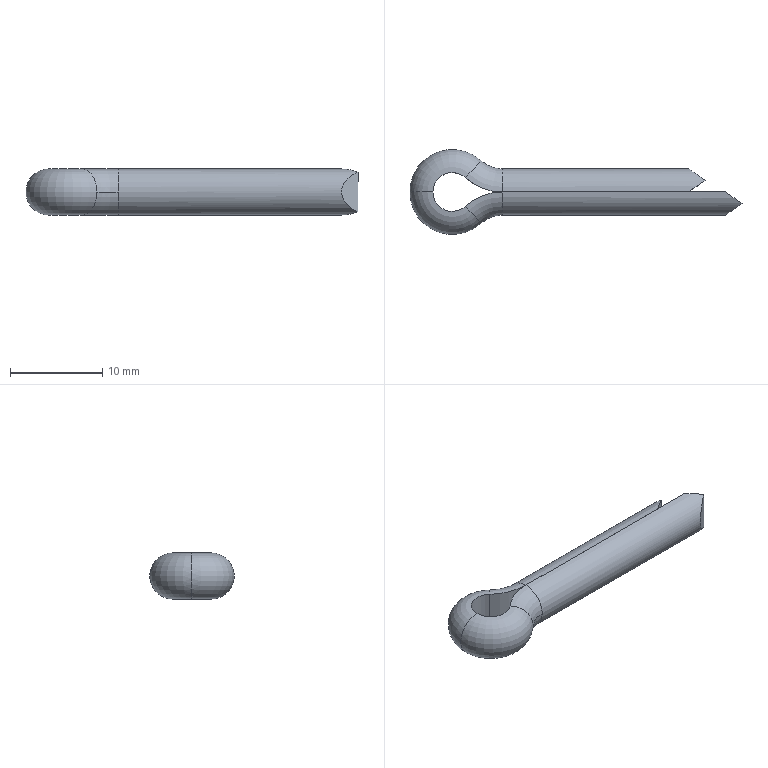Part | SolidWorks | features Cut 1, Sweep 1 | 1 solid | 17 faces | box 36 x 9.2 x 5 mm | volume 667.949 mm3 | torus 6 | plane 6 | cylinder 5 | commonest cylinder face diameters 5 x2 11.782 x2 4.204 x1
STEP:
#1=CARTESIAN_POINT('',(0.,2.5,0.));
#2=VERTEX_POINT('',#1);
#3=CARTESIAN_POINT('',(0.,0.002,2.5));
#4=VERTEX_POINT('',#3);
#5=CARTESIAN_POINT('',(0.,0.,0.));
#6=DIRECTION('',(1.,0.,0.));
#7=DIRECTION('',(0.,0.,-1.));
#8=AXIS2_PLACEMENT_3D('',#5,#6,#7);
#9=CIRCLE('',#8,2.5);
#10=EDGE_CURVE('',#2,#4,#9,.T.);
#11=ORIENTED_EDGE('',*,*,#10,.F.);
#12=CARTESIAN_POINT('',(-2.292,3.391,0.));
#13=VERTEX_POINT('',#12);
#14=CARTESIAN_POINT('',(0.,5.893,0.));
#15=DIRECTION('',(0.,0.,-1.));
#16=DIRECTION('',(-1.,0.,0.));
#17=AXIS2_PLACEMENT_3D('',#14,#15,#16);
#18=CIRCLE('',#17,3.393);
#19=EDGE_CURVE('',#2,#13,#18,.T.);
#20=ORIENTED_EDGE('',*,*,#19,.T.);
#21=CARTESIAN_POINT('',(-3.98,1.55,2.5));
#22=VERTEX_POINT('',#21);
#23=CARTESIAN_POINT('',(-3.981,1.548,0.));
#24=DIRECTION('',(0.7373,-0.6756,0.));
#25=DIRECTION('',(0.,0.,-1.));
#26=AXIS2_PLACEMENT_3D('',#23,#24,#25);
#27=CIRCLE('',#26,2.5);
#28=EDGE_CURVE('',#13,#22,#27,.T.);
#29=ORIENTED_EDGE('',*,*,#28,.T.);
#30=CARTESIAN_POINT('',(0.,5.893,2.5));
#31=DIRECTION('',(0.,0.,-1.));
#32=DIRECTION('',(-1.,0.,0.));
#33=AXIS2_PLACEMENT_3D('',#30,#31,#32);
#34=CIRCLE('',#33,5.891);
#35=EDGE_CURVE('',#4,#22,#34,.T.);
#36=ORIENTED_EDGE('',*,*,#35,.F.);
#37=EDGE_LOOP('',(#11,#20,#29,#36));
#38=FACE_OUTER_BOUND('',#37,.T.);
#39=CARTESIAN_POINT('',(0.,5.893,0.));
#40=DIRECTION('',(0.,0.,-1.));
#41=DIRECTION('',(-1.,0.,0.));
#42=AXIS2_PLACEMENT_3D('',#39,#40,#41);
#43=TOROIDAL_SURFACE('',#42,5.893,2.5);
#44=ADVANCED_FACE('',(#38),#43,.T.);
#45=CARTESIAN_POINT('',(-2.292,-3.391,0.));
#46=VERTEX_POINT('',#45);
#47=CARTESIAN_POINT('',(-3.98,-1.55,2.5));
#48=VERTEX_POINT('',#47);
#49=CARTESIAN_POINT('',(-3.981,-1.548,0.));
#50=DIRECTION('',(-0.7373,-0.6756,0.));
#51=DIRECTION('',(0.,0.,-1.));
#52=AXIS2_PLACEMENT_3D('',#49,#50,#51);
#53=CIRCLE('',#52,2.5);
#54=EDGE_CURVE('',#46,#48,#53,.T.);
#55=ORIENTED_EDGE('',*,*,#54,.F.);
#56=CARTESIAN_POINT('',(0.,-2.5,0.));
#57=VERTEX_POINT('',#56);
#58=CARTESIAN_POINT('',(0.,-5.893,0.));
#59=DIRECTION('',(0.,0.,-1.));
#60=DIRECTION('',(-1.,0.,0.));
#61=AXIS2_PLACEMENT_3D('',#58,#59,#60);
#62=CIRCLE('',#61,3.393);
#63=EDGE_CURVE('',#46,#57,#62,.T.);
#64=ORIENTED_EDGE('',*,*,#63,.T.);
#65=CARTESIAN_POINT('',(0.,-0.002,2.5));
#66=VERTEX_POINT('',#65);
#67=CARTESIAN_POINT('',(0.,0.,0.));
#68=DIRECTION('',(-1.,0.,0.));
#69=DIRECTION('',(0.,0.,-1.));
#70=AXIS2_PLACEMENT_3D('',#67,#68,#69);
#71=CIRCLE('',#70,2.5);
#72=EDGE_CURVE('',#57,#66,#71,.T.);
#73=ORIENTED_EDGE('',*,*,#72,.T.);
#74=CARTESIAN_POINT('',(0.,-5.893,2.5));
#75=DIRECTION('',(0.,0.,-1.));
#76=DIRECTION('',(-1.,0.,0.));
#77=AXIS2_PLACEMENT_3D('',#74,#75,#76);
#78=CIRCLE('',#77,5.891);
#79=EDGE_CURVE('',#48,#66,#78,.T.);
#80=ORIENTED_EDGE('',*,*,#79,.F.);
#81=EDGE_LOOP('',(#55,#64,#73,#80));
#82=FACE_OUTER_BOUND('',#81,.T.);
#83=CARTESIAN_POINT('',(0.,-5.893,0.));
#84=DIRECTION('',(0.,0.,-1.));
#85=DIRECTION('',(-1.,0.,0.));
#86=AXIS2_PLACEMENT_3D('',#83,#84,#85);
#87=TOROIDAL_SURFACE('',#86,5.893,2.5);
#88=ADVANCED_FACE('',(#82),#87,.T.);
#89=CARTESIAN_POINT('',(-3.98,1.55,-2.5));
#90=VERTEX_POINT('',#89);
#91=CARTESIAN_POINT('',(-7.502,0.,-2.5));
#92=VERTEX_POINT('',#91);
#93=CARTESIAN_POINT('',(-5.4,0.,-2.5));
#94=DIRECTION('',(0.,0.,1.));
#95=DIRECTION('',(1.,0.,0.));
#96=AXIS2_PLACEMENT_3D('',#93,#94,#95);
#97=CIRCLE('',#96,2.102);
#98=EDGE_CURVE('',#90,#92,#97,.T.);
#99=ORIENTED_EDGE('',*,*,#98,.T.);
#100=CARTESIAN_POINT('',(-7.502,0.,2.5));
#101=VERTEX_POINT('',#100);
#102=CARTESIAN_POINT('',(-7.5,0.,0.));
#103=DIRECTION('',(0.,1.,0.));
#104=DIRECTION('',(-1.,0.,0.));
#105=AXIS2_PLACEMENT_3D('',#102,#103,#104);
#106=CIRCLE('',#105,2.5);
#107=EDGE_CURVE('',#92,#101,#106,.T.);
#108=ORIENTED_EDGE('',*,*,#107,.T.);
#109=CARTESIAN_POINT('',(-5.4,0.,2.5));
#110=DIRECTION('',(0.,0.,1.));
#111=DIRECTION('',(1.,0.,0.));
#112=AXIS2_PLACEMENT_3D('',#109,#110,#111);
#113=CIRCLE('',#112,2.102);
#114=EDGE_CURVE('',#22,#101,#113,.T.);
#115=ORIENTED_EDGE('',*,*,#114,.F.);
#116=ORIENTED_EDGE('',*,*,#28,.F.);
#117=CARTESIAN_POINT('',(-3.981,1.548,0.));
#118=DIRECTION('',(0.7373,-0.6756,0.));
#119=DIRECTION('',(0.,0.,-1.));
#120=AXIS2_PLACEMENT_3D('',#117,#118,#119);
#121=CIRCLE('',#120,2.5);
#122=EDGE_CURVE('',#90,#13,#121,.T.);
#123=ORIENTED_EDGE('',*,*,#122,.F.);
#124=EDGE_LOOP('',(#99,#108,#115,#116,#123));
#125=FACE_OUTER_BOUND('',#124,.T.);
#126=CARTESIAN_POINT('',(-5.4,0.,0.));
#127=DIRECTION('',(0.,0.,1.));
#128=DIRECTION('',(1.,0.,0.));
#129=AXIS2_PLACEMENT_3D('',#126,#127,#128);
#130=TOROIDAL_SURFACE('',#129,2.1,2.5);
#131=ADVANCED_FACE('',(#125),#130,.T.);
#132=CARTESIAN_POINT('',(24.208,-0.002,2.5));
#133=VERTEX_POINT('',#132);
#134=CARTESIAN_POINT('',(0.,-0.002,2.5));
#135=DIRECTION('',(1.,0.,0.));
#136=VECTOR('',#135,1000.);
#137=LINE('',#134,#136);
#138=EDGE_CURVE('',#66,#133,#137,.T.);
#139=ORIENTED_EDGE('',*,*,#138,.T.);
#140=CARTESIAN_POINT('',(24.208,-0.002,-2.5));
#141=VERTEX_POINT('',#140);
#142=CARTESIAN_POINT('',(24.208,-0.002,2.5));
#143=DIRECTION('',(0.,0.,-1.));
#144=VECTOR('',#143,1000.);
#145=LINE('',#142,#144);
#146=EDGE_CURVE('',#133,#141,#145,.T.);
#147=ORIENTED_EDGE('',*,*,#146,.T.);
#148=CARTESIAN_POINT('',(0.,-0.002,-2.5));
#149=VERTEX_POINT('',#148);
#150=CARTESIAN_POINT('',(0.,-0.002,-2.5));
#151=DIRECTION('',(1.,0.,0.));
#152=VECTOR('',#151,1000.);
#153=LINE('',#150,#152);
#154=EDGE_CURVE('',#149,#141,#153,.T.);
#155=ORIENTED_EDGE('',*,*,#154,.F.);
#156=CARTESIAN_POINT('',(0.,-0.002,2.5));
#157=DIRECTION('',(0.,0.,-1.));
#158=VECTOR('',#157,1000.);
#159=LINE('',#156,#158);
#160=EDGE_CURVE('',#66,#149,#159,.T.);
#161=ORIENTED_EDGE('',*,*,#160,.F.);
#162=EDGE_LOOP('',(#139,#147,#155,#161));
#163=FACE_OUTER_BOUND('',#162,.T.);
#164=CARTESIAN_POINT('',(0.,-0.002,2.5));
#165=DIRECTION('',(0.,-1.,0.));
#166=DIRECTION('',(1.,0.,0.));
#167=AXIS2_PLACEMENT_3D('',#164,#165,#166);
#168=PLANE('',#167);
#169=ADVANCED_FACE('',(#163),#168,.F.);
#170=CARTESIAN_POINT('',(26.,-1.251,-2.164));
#171=VERTEX_POINT('',#170);
#172=CARTESIAN_POINT('',(26.,-1.251,2.164));
#173=VERTEX_POINT('',#172);
#174=CARTESIAN_POINT('',(26.,-1.251,-2.164));
#175=CARTESIAN_POINT('',(23.337,-3.124,-1.082));
#176=CARTESIAN_POINT('',(23.337,-3.124,1.082));
#177=CARTESIAN_POINT('',(26.,-1.251,2.164));
#178=(BOUNDED_CURVE()B_SPLINE_CURVE(3,(#174,#175,#176,#177),.UNSPECIFIED.,.F.,.T.)B_SPLINE_CURVE_WITH_KNOTS((4,4),(2.095,4.188),.UNSPECIFIED.)CURVE()GEOMETRIC_REPRESENTATION_ITEM()RATIONAL_B_SPLINE_CURVE((1.,0.6669,0.6669,1.))REPRESENTATION_ITEM(''));
#179=EDGE_CURVE('',#171,#173,#178,.T.);
#180=ORIENTED_EDGE('',*,*,#179,.T.);
#181=CARTESIAN_POINT('',(26.,-1.251,2.164));
#182=CARTESIAN_POINT('',(25.452,-0.8691,2.385));
#183=CARTESIAN_POINT('',(24.841,-0.4431,2.5));
#184=CARTESIAN_POINT('',(24.208,-0.002,2.5));
#185=(BOUNDED_CURVE()B_SPLINE_CURVE(3,(#181,#182,#183,#184),.UNSPECIFIED.,.F.,.F.)B_SPLINE_CURVE_WITH_KNOTS((4,4),(1.047,1.57),.UNSPECIFIED.)CURVE()GEOMETRIC_REPRESENTATION_ITEM()RATIONAL_B_SPLINE_CURVE((1.,0.9773,0.9773,1.))REPRESENTATION_ITEM(''));
#186=EDGE_CURVE('',#173,#133,#185,.T.);
#187=ORIENTED_EDGE('',*,*,#186,.T.);
#188=ORIENTED_EDGE('',*,*,#138,.F.);
#189=ORIENTED_EDGE('',*,*,#72,.F.);
#190=CARTESIAN_POINT('',(0.,0.,0.));
#191=DIRECTION('',(-1.,0.,0.));
#192=DIRECTION('',(0.,0.,-1.));
#193=AXIS2_PLACEMENT_3D('',#190,#191,#192);
#194=CIRCLE('',#193,2.5);
#195=EDGE_CURVE('',#149,#57,#194,.T.);
#196=ORIENTED_EDGE('',*,*,#195,.F.);
#197=ORIENTED_EDGE('',*,*,#154,.T.);
#198=CARTESIAN_POINT('',(24.208,-0.002,-2.5));
#199=CARTESIAN_POINT('',(24.841,-0.4431,-2.5));
#200=CARTESIAN_POINT('',(25.452,-0.8691,-2.385));
#201=CARTESIAN_POINT('',(26.,-1.251,-2.164));
#202=(BOUNDED_CURVE()B_SPLINE_CURVE(3,(#198,#199,#200,#201),.UNSPECIFIED.,.F.,.T.)B_SPLINE_CURVE_WITH_KNOTS((4,4),(4.713,5.236),.UNSPECIFIED.)CURVE()GEOMETRIC_REPRESENTATION_ITEM()RATIONAL_B_SPLINE_CURVE((1.,0.9773,0.9773,1.))REPRESENTATION_ITEM(''));
#203=EDGE_CURVE('',#141,#171,#202,.T.);
#204=ORIENTED_EDGE('',*,*,#203,.T.);
#205=EDGE_LOOP('',(#180,#187,#188,#189,#196,#197,#204));
#206=FACE_OUTER_BOUND('',#205,.T.);
#207=CARTESIAN_POINT('',(0.,0.,0.));
#208=DIRECTION('',(1.,0.,0.));
#209=DIRECTION('',(0.,1.,0.));
#210=AXIS2_PLACEMENT_3D('',#207,#208,#209);
#211=CYLINDRICAL_SURFACE('',#210,2.5);
#212=ADVANCED_FACE('',(#206),#211,.T.);
#213=CARTESIAN_POINT('',(-3.98,-1.55,-2.5));
#214=VERTEX_POINT('',#213);
#215=CARTESIAN_POINT('',(-3.98,-1.55,2.5));
#216=DIRECTION('',(0.,0.,-1.));
#217=VECTOR('',#216,1000.);
#218=LINE('',#215,#217);
#219=EDGE_CURVE('',#48,#214,#218,.T.);
#220=ORIENTED_EDGE('',*,*,#219,.F.);
#221=ORIENTED_EDGE('',*,*,#79,.T.);
#222=ORIENTED_EDGE('',*,*,#160,.T.);
#223=CARTESIAN_POINT('',(0.,-5.893,-2.5));
#224=DIRECTION('',(0.,0.,-1.));
#225=DIRECTION('',(-1.,0.,0.));
#226=AXIS2_PLACEMENT_3D('',#223,#224,#225);
#227=CIRCLE('',#226,5.891);
#228=EDGE_CURVE('',#214,#149,#227,.T.);
#229=ORIENTED_EDGE('',*,*,#228,.F.);
#230=EDGE_LOOP('',(#220,#221,#222,#229));
#231=FACE_OUTER_BOUND('',#230,.T.);
#232=CARTESIAN_POINT('',(0.,-5.893,0.));
#233=DIRECTION('',(0.,0.,-1.));
#234=DIRECTION('',(-1.,0.,0.));
#235=AXIS2_PLACEMENT_3D('',#232,#233,#234);
#236=CYLINDRICAL_SURFACE('',#235,5.891);
#237=ADVANCED_FACE('',(#231),#236,.T.);
#238=ORIENTED_EDGE('',*,*,#63,.F.);
#239=CARTESIAN_POINT('',(-3.981,-1.548,0.));
#240=DIRECTION('',(-0.7373,-0.6756,0.));
#241=DIRECTION('',(0.,0.,-1.));
#242=AXIS2_PLACEMENT_3D('',#239,#240,#241);
#243=CIRCLE('',#242,2.5);
#244=EDGE_CURVE('',#214,#46,#243,.T.);
#245=ORIENTED_EDGE('',*,*,#244,.F.);
#246=ORIENTED_EDGE('',*,*,#228,.T.);
#247=ORIENTED_EDGE('',*,*,#195,.T.);
#248=EDGE_LOOP('',(#238,#245,#246,#247));
#249=FACE_OUTER_BOUND('',#248,.T.);
#250=CARTESIAN_POINT('',(0.,-5.893,0.));
#251=DIRECTION('',(0.,0.,-1.));
#252=DIRECTION('',(-1.,0.,0.));
#253=AXIS2_PLACEMENT_3D('',#250,#251,#252);
#254=TOROIDAL_SURFACE('',#253,5.893,2.5);
#255=ADVANCED_FACE('',(#249),#254,.T.);
#256=CARTESIAN_POINT('',(-3.98,1.55,2.5));
#257=DIRECTION('',(0.,0.,-1.));
#258=VECTOR('',#257,1000.);
#259=LINE('',#256,#258);
#260=EDGE_CURVE('',#22,#90,#259,.T.);
#261=ORIENTED_EDGE('',*,*,#260,.F.);
#262=ORIENTED_EDGE('',*,*,#114,.T.);
#263=CARTESIAN_POINT('',(-5.4,0.,2.5));
#264=DIRECTION('',(0.,0.,1.));
#265=DIRECTION('',(1.,0.,0.));
#266=AXIS2_PLACEMENT_3D('',#263,#264,#265);
#267=CIRCLE('',#266,2.102);
#268=EDGE_CURVE('',#101,#48,#267,.T.);
#269=ORIENTED_EDGE('',*,*,#268,.T.);
#270=ORIENTED_EDGE('',*,*,#219,.T.);
#271=CARTESIAN_POINT('',(-5.4,0.,-2.5));
#272=DIRECTION('',(0.,0.,1.));
#273=DIRECTION('',(1.,0.,0.));
#274=AXIS2_PLACEMENT_3D('',#271,#272,#273);
#275=CIRCLE('',#274,2.102);
#276=EDGE_CURVE('',#92,#214,#275,.T.);
#277=ORIENTED_EDGE('',*,*,#276,.F.);
#278=ORIENTED_EDGE('',*,*,#98,.F.);
#279=EDGE_LOOP('',(#261,#262,#269,#270,#277,#278));
#280=FACE_OUTER_BOUND('',#279,.T.);
#281=CARTESIAN_POINT('',(-5.4,0.,0.));
#282=DIRECTION('',(0.,0.,1.));
#283=DIRECTION('',(1.,0.,0.));
#284=AXIS2_PLACEMENT_3D('',#281,#282,#283);
#285=CYLINDRICAL_SURFACE('',#284,2.102);
#286=ADVANCED_FACE('',(#280),#285,.F.);
#287=ORIENTED_EDGE('',*,*,#107,.F.);
#288=ORIENTED_EDGE('',*,*,#276,.T.);
#289=ORIENTED_EDGE('',*,*,#244,.T.);
#290=ORIENTED_EDGE('',*,*,#54,.T.);
#291=ORIENTED_EDGE('',*,*,#268,.F.);
#292=EDGE_LOOP('',(#287,#288,#289,#290,#291));
#293=FACE_OUTER_BOUND('',#292,.T.);
#294=CARTESIAN_POINT('',(-5.4,0.,0.));
#295=DIRECTION('',(0.,0.,1.));
#296=DIRECTION('',(1.,0.,0.));
#297=AXIS2_PLACEMENT_3D('',#294,#295,#296);
#298=TOROIDAL_SURFACE('',#297,2.1,2.5);
#299=ADVANCED_FACE('',(#293),#298,.T.);
#300=CARTESIAN_POINT('',(0.,0.002,-2.5));
#301=VERTEX_POINT('',#300);
#302=CARTESIAN_POINT('',(0.,0.002,2.5));
#303=DIRECTION('',(0.,0.,-1.));
#304=VECTOR('',#303,1000.);
#305=LINE('',#302,#304);
#306=EDGE_CURVE('',#4,#301,#305,.T.);
#307=ORIENTED_EDGE('',*,*,#306,.F.);
#308=ORIENTED_EDGE('',*,*,#35,.T.);
#309=ORIENTED_EDGE('',*,*,#260,.T.);
#310=CARTESIAN_POINT('',(0.,5.893,-2.5));
#311=DIRECTION('',(0.,0.,-1.));
#312=DIRECTION('',(-1.,0.,0.));
#313=AXIS2_PLACEMENT_3D('',#310,#311,#312);
#314=CIRCLE('',#313,5.891);
#315=EDGE_CURVE('',#301,#90,#314,.T.);
#316=ORIENTED_EDGE('',*,*,#315,.F.);
#317=EDGE_LOOP('',(#307,#308,#309,#316));
#318=FACE_OUTER_BOUND('',#317,.T.);
#319=CARTESIAN_POINT('',(0.,5.893,0.));
#320=DIRECTION('',(0.,0.,-1.));
#321=DIRECTION('',(-1.,0.,0.));
#322=AXIS2_PLACEMENT_3D('',#319,#320,#321);
#323=CYLINDRICAL_SURFACE('',#322,5.891);
#324=ADVANCED_FACE('',(#318),#323,.T.);
#325=ORIENTED_EDGE('',*,*,#19,.F.);
#326=CARTESIAN_POINT('',(0.,0.,0.));
#327=DIRECTION('',(1.,0.,0.));
#328=DIRECTION('',(0.,0.,-1.));
#329=AXIS2_PLACEMENT_3D('',#326,#327,#328);
#330=CIRCLE('',#329,2.5);
#331=EDGE_CURVE('',#301,#2,#330,.T.);
#332=ORIENTED_EDGE('',*,*,#331,.F.);
#333=ORIENTED_EDGE('',*,*,#315,.T.);
#334=ORIENTED_EDGE('',*,*,#122,.T.);
#335=EDGE_LOOP('',(#325,#332,#333,#334));
#336=FACE_OUTER_BOUND('',#335,.T.);
#337=CARTESIAN_POINT('',(0.,5.893,0.));
#338=DIRECTION('',(0.,0.,-1.));
#339=DIRECTION('',(-1.,0.,0.));
#340=AXIS2_PLACEMENT_3D('',#337,#338,#339);
#341=TOROIDAL_SURFACE('',#340,5.893,2.5);
#342=ADVANCED_FACE('',(#336),#341,.T.);
#343=CARTESIAN_POINT('',(22.,1.251,2.164));
#344=VERTEX_POINT('',#343);
#345=CARTESIAN_POINT('',(20.208,0.002,2.5));
#346=VERTEX_POINT('',#345);
#347=CARTESIAN_POINT('',(22.,1.251,2.164));
#348=CARTESIAN_POINT('',(21.452,0.8691,2.385));
#349=CARTESIAN_POINT('',(20.841,0.4431,2.5));
#350=CARTESIAN_POINT('',(20.208,0.002,2.5));
#351=(BOUNDED_CURVE()B_SPLINE_CURVE(3,(#347,#348,#349,#350),.UNSPECIFIED.,.F.,.F.)B_SPLINE_CURVE_WITH_KNOTS((4,4),(1.047,1.57),.UNSPECIFIED.)CURVE()GEOMETRIC_REPRESENTATION_ITEM()RATIONAL_B_SPLINE_CURVE((1.,0.9773,0.9773,1.))REPRESENTATION_ITEM(''));
#352=EDGE_CURVE('',#344,#346,#351,.T.);
#353=ORIENTED_EDGE('',*,*,#352,.F.);
#354=CARTESIAN_POINT('',(22.,1.251,-2.164));
#355=VERTEX_POINT('',#354);
#356=CARTESIAN_POINT('',(22.,1.251,-2.164));
#357=CARTESIAN_POINT('',(19.337,3.124,-1.082));
#358=CARTESIAN_POINT('',(19.337,3.124,1.082));
#359=CARTESIAN_POINT('',(22.,1.251,2.164));
#360=(BOUNDED_CURVE()B_SPLINE_CURVE(3,(#356,#357,#358,#359),.UNSPECIFIED.,.F.,.T.)B_SPLINE_CURVE_WITH_KNOTS((4,4),(2.095,4.188),.UNSPECIFIED.)CURVE()GEOMETRIC_REPRESENTATION_ITEM()RATIONAL_B_SPLINE_CURVE((1.,0.6669,0.6669,1.))REPRESENTATION_ITEM(''));
#361=EDGE_CURVE('',#355,#344,#360,.T.);
#362=ORIENTED_EDGE('',*,*,#361,.F.);
#363=CARTESIAN_POINT('',(20.208,0.002,-2.5));
#364=VERTEX_POINT('',#363);
#365=CARTESIAN_POINT('',(20.208,0.002,-2.5));
#366=CARTESIAN_POINT('',(20.841,0.4431,-2.5));
#367=CARTESIAN_POINT('',(21.452,0.8691,-2.385));
#368=CARTESIAN_POINT('',(22.,1.251,-2.164));
#369=(BOUNDED_CURVE()B_SPLINE_CURVE(3,(#365,#366,#367,#368),.UNSPECIFIED.,.F.,.F.)B_SPLINE_CURVE_WITH_KNOTS((4,4),(4.713,5.236),.UNSPECIFIED.)CURVE()GEOMETRIC_REPRESENTATION_ITEM()RATIONAL_B_SPLINE_CURVE((1.,0.9773,0.9773,1.))REPRESENTATION_ITEM(''));
#370=EDGE_CURVE('',#364,#355,#369,.T.);
#371=ORIENTED_EDGE('',*,*,#370,.F.);
#372=CARTESIAN_POINT('',(0.,0.002,-2.5));
#373=DIRECTION('',(1.,0.,0.));
#374=VECTOR('',#373,1000.);
#375=LINE('',#372,#374);
#376=EDGE_CURVE('',#301,#364,#375,.T.);
#377=ORIENTED_EDGE('',*,*,#376,.F.);
#378=ORIENTED_EDGE('',*,*,#331,.T.);
#379=ORIENTED_EDGE('',*,*,#10,.T.);
#380=CARTESIAN_POINT('',(0.,0.002,2.5));
#381=DIRECTION('',(1.,0.,0.));
#382=VECTOR('',#381,1000.);
#383=LINE('',#380,#382);
#384=EDGE_CURVE('',#4,#346,#383,.T.);
#385=ORIENTED_EDGE('',*,*,#384,.T.);
#386=EDGE_LOOP('',(#353,#362,#371,#377,#378,#379,#385));
#387=FACE_OUTER_BOUND('',#386,.T.);
#388=CARTESIAN_POINT('',(0.,0.,0.));
#389=DIRECTION('',(1.,0.,0.));
#390=DIRECTION('',(0.,0.,-1.));
#391=AXIS2_PLACEMENT_3D('',#388,#389,#390);
#392=CYLINDRICAL_SURFACE('',#391,2.5);
#393=ADVANCED_FACE('',(#387),#392,.T.);
#394=CARTESIAN_POINT('',(20.208,0.002,2.5));
#395=DIRECTION('',(0.,0.,-1.));
#396=VECTOR('',#395,1000.);
#397=LINE('',#394,#396);
#398=EDGE_CURVE('',#346,#364,#397,.T.);
#399=ORIENTED_EDGE('',*,*,#398,.F.);
#400=ORIENTED_EDGE('',*,*,#384,.F.);
#401=ORIENTED_EDGE('',*,*,#306,.T.);
#402=ORIENTED_EDGE('',*,*,#376,.T.);
#403=EDGE_LOOP('',(#399,#400,#401,#402));
#404=FACE_OUTER_BOUND('',#403,.T.);
#405=CARTESIAN_POINT('',(0.,0.002,2.5));
#406=DIRECTION('',(0.,-1.,0.));
#407=DIRECTION('',(0.,0.,-1.));
#408=AXIS2_PLACEMENT_3D('',#405,#406,#407);
#409=PLANE('',#408);
#410=ADVANCED_FACE('',(#404),#409,.T.);
#411=ORIENTED_EDGE('',*,*,#352,.T.);
#412=ORIENTED_EDGE('',*,*,#398,.T.);
#413=ORIENTED_EDGE('',*,*,#370,.T.);
#414=CARTESIAN_POINT('',(22.,1.251,-2.5));
#415=DIRECTION('',(0.,0.,1.));
#416=VECTOR('',#415,1000.);
#417=LINE('',#414,#416);
#418=EDGE_CURVE('',#355,#344,#417,.T.);
#419=ORIENTED_EDGE('',*,*,#418,.T.);
#420=EDGE_LOOP('',(#411,#412,#413,#419));
#421=FACE_OUTER_BOUND('',#420,.T.);
#422=CARTESIAN_POINT('',(22.,1.251,-2.5));
#423=DIRECTION('',(-0.5717,0.8204,0.));
#424=DIRECTION('',(-0.8204,-0.5717,0.));
#425=AXIS2_PLACEMENT_3D('',#422,#423,#424);
#426=PLANE('',#425);
#427=ADVANCED_FACE('',(#421),#426,.F.);
#428=ORIENTED_EDGE('',*,*,#361,.T.);
#429=ORIENTED_EDGE('',*,*,#418,.F.);
#430=EDGE_LOOP('',(#428,#429));
#431=FACE_OUTER_BOUND('',#430,.T.);
#432=CARTESIAN_POINT('',(22.,1.251,-2.5));
#433=DIRECTION('',(-0.5754,-0.8179,0.));
#434=DIRECTION('',(0.8179,-0.5754,0.));
#435=AXIS2_PLACEMENT_3D('',#432,#433,#434);
#436=PLANE('',#435);
#437=ADVANCED_FACE('',(#431),#436,.F.);
#438=CARTESIAN_POINT('',(26.,-1.251,-2.5));
#439=DIRECTION('',(0.,0.,1.));
#440=VECTOR('',#439,1000.);
#441=LINE('',#438,#440);
#442=EDGE_CURVE('',#171,#173,#441,.T.);
#443=ORIENTED_EDGE('',*,*,#442,.T.);
#444=ORIENTED_EDGE('',*,*,#179,.F.);
#445=EDGE_LOOP('',(#443,#444));
#446=FACE_OUTER_BOUND('',#445,.T.);
#447=CARTESIAN_POINT('',(26.,-1.251,-2.5));
#448=DIRECTION('',(-0.5754,0.8179,0.));
#449=DIRECTION('',(-0.8179,-0.5754,0.));
#450=AXIS2_PLACEMENT_3D('',#447,#448,#449);
#451=PLANE('',#450);
#452=ADVANCED_FACE('',(#446),#451,.F.);
#453=ORIENTED_EDGE('',*,*,#442,.F.);
#454=ORIENTED_EDGE('',*,*,#203,.F.);
#455=ORIENTED_EDGE('',*,*,#146,.F.);
#456=ORIENTED_EDGE('',*,*,#186,.F.);
#457=EDGE_LOOP('',(#453,#454,#455,#456));
#458=FACE_OUTER_BOUND('',#457,.T.);
#459=CARTESIAN_POINT('',(26.,-1.251,-2.5));
#460=DIRECTION('',(-0.5717,-0.8204,0.));
#461=DIRECTION('',(0.8204,-0.5717,0.));
#462=AXIS2_PLACEMENT_3D('',#459,#460,#461);
#463=PLANE('',#462);
#464=ADVANCED_FACE('',(#458),#463,.F.);
#465=CLOSED_SHELL('',(#44,#88,#131,#169,#212,#237,#255,#286,#299,#324,#342,#393,#410,#427,#437,#452,#464));
#466=MANIFOLD_SOLID_BREP('',#465);
#467=CARTESIAN_POINT('',(0.,0.,0.));
#468=DIRECTION('',(0.,0.,1.));
#469=DIRECTION('',(1.,0.,0.));
#470=AXIS2_PLACEMENT_3D('',#467,#468,#469);
#471=(LENGTH_UNIT()NAMED_UNIT(*)SI_UNIT(.MILLI.,.METRE.));
#472=UNCERTAINTY_MEASURE_WITH_UNIT(LENGTH_MEASURE(0.00001),#471,'','');
#473=(NAMED_UNIT(*)PLANE_ANGLE_UNIT()SI_UNIT($,.RADIAN.));
#474=(NAMED_UNIT(*)SI_UNIT($,.STERADIAN.)SOLID_ANGLE_UNIT());
#475=(GEOMETRIC_REPRESENTATION_CONTEXT(3)GLOBAL_UNCERTAINTY_ASSIGNED_CONTEXT((#472))GLOBAL_UNIT_ASSIGNED_CONTEXT((#471,#473,#474))REPRESENTATION_CONTEXT('',''));
#476=ADVANCED_BREP_SHAPE_REPRESENTATION('',(#466,#470),#475);